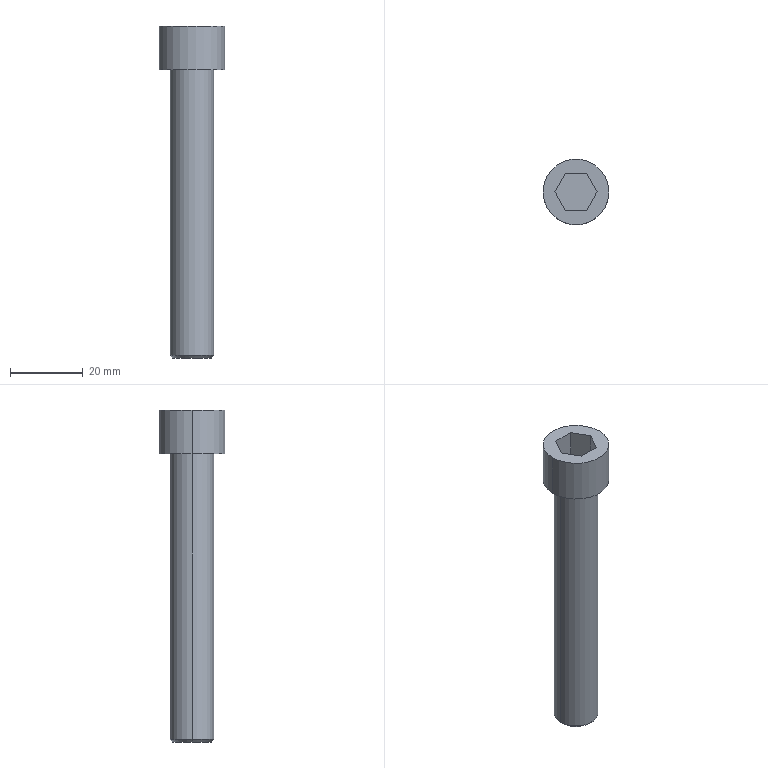Part | Creo | 1 solid | 16 faces | box 18 x 18 x 91 mm | volume 11293 mm3 | plane 10 | cylinder 4 | cone 2 | commonest cylinder face diameters 12 x2 18 x2
STEP:
#1=CARTESIAN_POINT('',(0.,0.,0.));
#2=DIRECTION('',(0.,0.,1.));
#3=DIRECTION('',(1.,0.,0.));
#4=AXIS2_PLACEMENT_3D('',#1,#2,#3);
#5=CARTESIAN_POINT('',(190.927,150.543,206.956));
#6=VERTEX_POINT('',#5);
#7=CARTESIAN_POINT('',(202.927,150.543,206.956));
#8=VERTEX_POINT('',#7);
#9=CARTESIAN_POINT('',(196.927,150.543,206.956));
#10=DIRECTION('',(0.,0.,-1.));
#11=DIRECTION('',(-1.,0.,0.));
#12=AXIS2_PLACEMENT_3D('',#9,#10,#11);
#13=CIRCLE('',#12,6.);
#14=EDGE_CURVE('',#6,#8,#13,.T.);
#15=ORIENTED_EDGE('',*,*,#14,.T.);
#16=CARTESIAN_POINT('',(202.927,150.543,285.245));
#17=VERTEX_POINT('',#16);
#18=CARTESIAN_POINT('',(202.927,150.543,285.245));
#19=DIRECTION('',(0.,0.,-1.));
#20=VECTOR('',#19,78.29);
#21=LINE('',#18,#20);
#22=EDGE_CURVE('',#17,#8,#21,.T.);
#23=ORIENTED_EDGE('',*,*,#22,.F.);
#24=CARTESIAN_POINT('',(190.927,150.543,285.245));
#25=VERTEX_POINT('',#24);
#26=CARTESIAN_POINT('',(196.927,150.543,285.245));
#27=DIRECTION('',(0.,0.,1.));
#28=DIRECTION('',(1.,0.,0.));
#29=AXIS2_PLACEMENT_3D('',#26,#27,#28);
#30=CIRCLE('',#29,6.);
#31=EDGE_CURVE('',#17,#25,#30,.T.);
#32=ORIENTED_EDGE('',*,*,#31,.T.);
#33=CARTESIAN_POINT('',(190.927,150.543,285.245));
#34=DIRECTION('',(0.,0.,-1.));
#35=VECTOR('',#34,78.29);
#36=LINE('',#33,#35);
#37=EDGE_CURVE('',#25,#6,#36,.T.);
#38=ORIENTED_EDGE('',*,*,#37,.T.);
#39=EDGE_LOOP('',(#15,#23,#32,#38));
#40=FACE_OUTER_BOUND('',#39,.F.);
#41=CARTESIAN_POINT('',(196.927,150.543,285.245));
#42=DIRECTION('',(0.,0.,-1.));
#43=DIRECTION('',(-1.,0.,0.));
#44=AXIS2_PLACEMENT_3D('',#41,#42,#43);
#45=CYLINDRICAL_SURFACE('',#44,6.);
#46=ADVANCED_FACE('',(#40),#45,.T.);
#47=CARTESIAN_POINT('',(191.637,150.543,206.245));
#48=VERTEX_POINT('',#47);
#49=CARTESIAN_POINT('',(202.216,150.543,206.245));
#50=VERTEX_POINT('',#49);
#51=CARTESIAN_POINT('',(196.927,150.543,206.245));
#52=DIRECTION('',(0.,0.,-1.));
#53=DIRECTION('',(-1.,0.,0.));
#54=AXIS2_PLACEMENT_3D('',#51,#52,#53);
#55=CIRCLE('',#54,5.29);
#56=EDGE_CURVE('',#48,#50,#55,.T.);
#57=ORIENTED_EDGE('',*,*,#56,.T.);
#58=CARTESIAN_POINT('',(202.216,150.543,206.245));
#59=DIRECTION('',(0.7071,0.,0.7071));
#60=VECTOR('',#59,1.005);
#61=LINE('',#58,#60);
#62=EDGE_CURVE('',#50,#8,#61,.T.);
#63=ORIENTED_EDGE('',*,*,#62,.T.);
#64=ORIENTED_EDGE('',*,*,#14,.F.);
#65=CARTESIAN_POINT('',(191.637,150.543,206.245));
#66=DIRECTION('',(-0.7071,0.,0.7071));
#67=VECTOR('',#66,1.005);
#68=LINE('',#65,#67);
#69=EDGE_CURVE('',#48,#6,#68,.T.);
#70=ORIENTED_EDGE('',*,*,#69,.F.);
#71=EDGE_LOOP('',(#57,#63,#64,#70));
#72=FACE_OUTER_BOUND('',#71,.F.);
#73=CARTESIAN_POINT('',(196.927,150.543,206.601));
#74=DIRECTION('',(0.,0.,1.));
#75=DIRECTION('',(1.,0.,0.));
#76=AXIS2_PLACEMENT_3D('',#73,#74,#75);
#77=CONICAL_SURFACE('',#76,5.645,45.);
#78=ADVANCED_FACE('',(#72),#77,.T.);
#79=CARTESIAN_POINT('',(196.927,150.543,206.245));
#80=DIRECTION('',(0.,0.,-1.));
#81=DIRECTION('',(1.,0.,0.));
#82=AXIS2_PLACEMENT_3D('',#79,#80,#81);
#83=CIRCLE('',#82,5.29);
#84=EDGE_CURVE('',#50,#48,#83,.T.);
#85=ORIENTED_EDGE('',*,*,#84,.F.);
#86=ORIENTED_EDGE('',*,*,#56,.F.);
#87=EDGE_LOOP('',(#85,#86));
#88=FACE_OUTER_BOUND('',#87,.F.);
#89=CARTESIAN_POINT('',(196.927,150.543,206.245));
#90=DIRECTION('',(0.,0.,1.));
#91=DIRECTION('',(1.,0.,0.));
#92=AXIS2_PLACEMENT_3D('',#89,#90,#91);
#93=PLANE('',#92);
#94=ADVANCED_FACE('',(#88),#93,.F.);
#95=ORIENTED_EDGE('',*,*,#84,.T.);
#96=ORIENTED_EDGE('',*,*,#69,.T.);
#97=CARTESIAN_POINT('',(196.927,150.543,206.956));
#98=DIRECTION('',(0.,0.,-1.));
#99=DIRECTION('',(1.,0.,0.));
#100=AXIS2_PLACEMENT_3D('',#97,#98,#99);
#101=CIRCLE('',#100,6.);
#102=EDGE_CURVE('',#8,#6,#101,.T.);
#103=ORIENTED_EDGE('',*,*,#102,.F.);
#104=ORIENTED_EDGE('',*,*,#62,.F.);
#105=EDGE_LOOP('',(#95,#96,#103,#104));
#106=FACE_OUTER_BOUND('',#105,.F.);
#107=CARTESIAN_POINT('',(196.927,150.543,206.601));
#108=DIRECTION('',(0.,0.,1.));
#109=DIRECTION('',(1.,0.,0.));
#110=AXIS2_PLACEMENT_3D('',#107,#108,#109);
#111=CONICAL_SURFACE('',#110,5.645,45.);
#112=ADVANCED_FACE('',(#106),#111,.T.);
#113=ORIENTED_EDGE('',*,*,#102,.T.);
#114=ORIENTED_EDGE('',*,*,#37,.F.);
#115=CARTESIAN_POINT('',(196.927,150.543,285.245));
#116=DIRECTION('',(0.,0.,1.));
#117=DIRECTION('',(-1.,0.,0.));
#118=AXIS2_PLACEMENT_3D('',#115,#116,#117);
#119=CIRCLE('',#118,6.);
#120=EDGE_CURVE('',#25,#17,#119,.T.);
#121=ORIENTED_EDGE('',*,*,#120,.T.);
#122=ORIENTED_EDGE('',*,*,#22,.T.);
#123=EDGE_LOOP('',(#113,#114,#121,#122));
#124=FACE_OUTER_BOUND('',#123,.F.);
#125=CARTESIAN_POINT('',(196.927,150.543,285.245));
#126=DIRECTION('',(0.,0.,-1.));
#127=DIRECTION('',(-1.,0.,0.));
#128=AXIS2_PLACEMENT_3D('',#125,#126,#127);
#129=CYLINDRICAL_SURFACE('',#128,6.);
#130=ADVANCED_FACE('',(#124),#129,.T.);
#131=CARTESIAN_POINT('',(205.927,150.543,285.245));
#132=VERTEX_POINT('',#131);
#133=CARTESIAN_POINT('',(187.927,150.543,285.245));
#134=VERTEX_POINT('',#133);
#135=CARTESIAN_POINT('',(196.927,150.543,285.245));
#136=DIRECTION('',(0.,0.,-1.));
#137=DIRECTION('',(1.,0.,0.));
#138=AXIS2_PLACEMENT_3D('',#135,#136,#137);
#139=CIRCLE('',#138,9.);
#140=EDGE_CURVE('',#132,#134,#139,.T.);
#141=ORIENTED_EDGE('',*,*,#140,.F.);
#142=CARTESIAN_POINT('',(196.927,150.543,285.245));
#143=DIRECTION('',(0.,0.,-1.));
#144=DIRECTION('',(-1.,0.,0.));
#145=AXIS2_PLACEMENT_3D('',#142,#143,#144);
#146=CIRCLE('',#145,9.);
#147=EDGE_CURVE('',#134,#132,#146,.T.);
#148=ORIENTED_EDGE('',*,*,#147,.F.);
#149=EDGE_LOOP('',(#141,#148));
#150=FACE_OUTER_BOUND('',#149,.F.);
#151=ORIENTED_EDGE('',*,*,#31,.F.);
#152=ORIENTED_EDGE('',*,*,#120,.F.);
#153=EDGE_LOOP('',(#151,#152));
#154=FACE_BOUND('',#153,.F.);
#155=CARTESIAN_POINT('',(196.927,150.543,285.245));
#156=DIRECTION('',(0.,0.,-1.));
#157=DIRECTION('',(-1.,0.,0.));
#158=AXIS2_PLACEMENT_3D('',#155,#156,#157);
#159=PLANE('',#158);
#160=ADVANCED_FACE('',(#150,#154),#159,.T.);
#161=CARTESIAN_POINT('',(187.927,150.543,297.245));
#162=VERTEX_POINT('',#161);
#163=CARTESIAN_POINT('',(205.927,150.543,297.245));
#164=VERTEX_POINT('',#163);
#165=CARTESIAN_POINT('',(196.927,150.543,297.245));
#166=DIRECTION('',(0.,0.,1.));
#167=DIRECTION('',(-1.,0.,0.));
#168=AXIS2_PLACEMENT_3D('',#165,#166,#167);
#169=CIRCLE('',#168,9.);
#170=EDGE_CURVE('',#162,#164,#169,.T.);
#171=ORIENTED_EDGE('',*,*,#170,.T.);
#172=CARTESIAN_POINT('',(205.927,150.543,285.245));
#173=DIRECTION('',(0.,0.,1.));
#174=VECTOR('',#173,12.);
#175=LINE('',#172,#174);
#176=EDGE_CURVE('',#132,#164,#175,.T.);
#177=ORIENTED_EDGE('',*,*,#176,.F.);
#178=ORIENTED_EDGE('',*,*,#140,.T.);
#179=CARTESIAN_POINT('',(187.927,150.543,285.245));
#180=DIRECTION('',(0.,0.,1.));
#181=VECTOR('',#180,12.);
#182=LINE('',#179,#181);
#183=EDGE_CURVE('',#134,#162,#182,.T.);
#184=ORIENTED_EDGE('',*,*,#183,.T.);
#185=EDGE_LOOP('',(#171,#177,#178,#184));
#186=FACE_OUTER_BOUND('',#185,.F.);
#187=CARTESIAN_POINT('',(196.927,150.543,285.245));
#188=DIRECTION('',(0.,0.,1.));
#189=DIRECTION('',(1.,0.,0.));
#190=AXIS2_PLACEMENT_3D('',#187,#188,#189);
#191=CYLINDRICAL_SURFACE('',#190,9.);
#192=ADVANCED_FACE('',(#186),#191,.T.);
#193=CARTESIAN_POINT('',(196.927,150.543,297.245));
#194=DIRECTION('',(0.,0.,1.));
#195=DIRECTION('',(1.,0.,0.));
#196=AXIS2_PLACEMENT_3D('',#193,#194,#195);
#197=CIRCLE('',#196,9.);
#198=EDGE_CURVE('',#164,#162,#197,.T.);
#199=ORIENTED_EDGE('',*,*,#198,.F.);
#200=ORIENTED_EDGE('',*,*,#170,.F.);
#201=EDGE_LOOP('',(#199,#200));
#202=FACE_OUTER_BOUND('',#201,.F.);
#203=CARTESIAN_POINT('',(199.813,145.543,297.245));
#204=VERTEX_POINT('',#203);
#205=CARTESIAN_POINT('',(194.04,145.543,297.245));
#206=VERTEX_POINT('',#205);
#207=CARTESIAN_POINT('',(199.813,145.543,297.245));
#208=DIRECTION('',(-1.,0.,0.));
#209=VECTOR('',#208,5.774);
#210=LINE('',#207,#209);
#211=EDGE_CURVE('',#204,#206,#210,.T.);
#212=ORIENTED_EDGE('',*,*,#211,.F.);
#213=CARTESIAN_POINT('',(202.7,150.543,297.245));
#214=VERTEX_POINT('',#213);
#215=CARTESIAN_POINT('',(202.7,150.543,297.245));
#216=DIRECTION('',(-0.5,-0.866,0.));
#217=VECTOR('',#216,5.774);
#218=LINE('',#215,#217);
#219=EDGE_CURVE('',#214,#204,#218,.T.);
#220=ORIENTED_EDGE('',*,*,#219,.F.);
#221=CARTESIAN_POINT('',(199.813,155.543,297.245));
#222=VERTEX_POINT('',#221);
#223=CARTESIAN_POINT('',(199.813,155.543,297.245));
#224=DIRECTION('',(0.5,-0.866,0.));
#225=VECTOR('',#224,5.774);
#226=LINE('',#223,#225);
#227=EDGE_CURVE('',#222,#214,#226,.T.);
#228=ORIENTED_EDGE('',*,*,#227,.F.);
#229=CARTESIAN_POINT('',(194.04,155.543,297.245));
#230=VERTEX_POINT('',#229);
#231=CARTESIAN_POINT('',(194.04,155.543,297.245));
#232=DIRECTION('',(1.,0.,0.));
#233=VECTOR('',#232,5.774);
#234=LINE('',#231,#233);
#235=EDGE_CURVE('',#230,#222,#234,.T.);
#236=ORIENTED_EDGE('',*,*,#235,.F.);
#237=CARTESIAN_POINT('',(191.153,150.543,297.245));
#238=VERTEX_POINT('',#237);
#239=CARTESIAN_POINT('',(191.153,150.543,297.245));
#240=DIRECTION('',(0.5,0.866,0.));
#241=VECTOR('',#240,5.774);
#242=LINE('',#239,#241);
#243=EDGE_CURVE('',#238,#230,#242,.T.);
#244=ORIENTED_EDGE('',*,*,#243,.F.);
#245=CARTESIAN_POINT('',(194.04,145.543,297.245));
#246=DIRECTION('',(-0.5,0.866,0.));
#247=VECTOR('',#246,5.774);
#248=LINE('',#245,#247);
#249=EDGE_CURVE('',#206,#238,#248,.T.);
#250=ORIENTED_EDGE('',*,*,#249,.F.);
#251=EDGE_LOOP('',(#212,#220,#228,#236,#244,#250));
#252=FACE_BOUND('',#251,.F.);
#253=CARTESIAN_POINT('',(196.927,150.543,297.245));
#254=DIRECTION('',(0.,0.,1.));
#255=DIRECTION('',(1.,0.,0.));
#256=AXIS2_PLACEMENT_3D('',#253,#254,#255);
#257=PLANE('',#256);
#258=ADVANCED_FACE('',(#202,#252),#257,.T.);
#259=ORIENTED_EDGE('',*,*,#211,.T.);
#260=CARTESIAN_POINT('',(194.04,145.543,289.325));
#261=VERTEX_POINT('',#260);
#262=CARTESIAN_POINT('',(194.04,145.543,297.245));
#263=DIRECTION('',(0.,0.,-1.));
#264=VECTOR('',#263,7.92);
#265=LINE('',#262,#264);
#266=EDGE_CURVE('',#206,#261,#265,.T.);
#267=ORIENTED_EDGE('',*,*,#266,.T.);
#268=CARTESIAN_POINT('',(199.813,145.543,289.325));
#269=VERTEX_POINT('',#268);
#270=CARTESIAN_POINT('',(199.813,145.543,289.325));
#271=DIRECTION('',(-1.,0.,0.));
#272=VECTOR('',#271,5.774);
#273=LINE('',#270,#272);
#274=EDGE_CURVE('',#269,#261,#273,.T.);
#275=ORIENTED_EDGE('',*,*,#274,.F.);
#276=CARTESIAN_POINT('',(199.813,145.543,297.245));
#277=DIRECTION('',(0.,0.,-1.));
#278=VECTOR('',#277,7.92);
#279=LINE('',#276,#278);
#280=EDGE_CURVE('',#204,#269,#279,.T.);
#281=ORIENTED_EDGE('',*,*,#280,.F.);
#282=EDGE_LOOP('',(#259,#267,#275,#281));
#283=FACE_OUTER_BOUND('',#282,.F.);
#284=CARTESIAN_POINT('',(194.04,145.543,289.325));
#285=DIRECTION('',(0.,-1.,0.));
#286=DIRECTION('',(0.,0.,-1.));
#287=AXIS2_PLACEMENT_3D('',#284,#285,#286);
#288=PLANE('',#287);
#289=ADVANCED_FACE('',(#283),#288,.F.);
#290=ORIENTED_EDGE('',*,*,#249,.T.);
#291=CARTESIAN_POINT('',(191.153,150.543,289.325));
#292=VERTEX_POINT('',#291);
#293=CARTESIAN_POINT('',(191.153,150.543,297.245));
#294=DIRECTION('',(0.,0.,-1.));
#295=VECTOR('',#294,7.92);
#296=LINE('',#293,#295);
#297=EDGE_CURVE('',#238,#292,#296,.T.);
#298=ORIENTED_EDGE('',*,*,#297,.T.);
#299=CARTESIAN_POINT('',(191.153,150.543,289.325));
#300=DIRECTION('',(0.5,-0.866,0.));
#301=VECTOR('',#300,5.774);
#302=LINE('',#299,#301);
#303=EDGE_CURVE('',#292,#261,#302,.T.);
#304=ORIENTED_EDGE('',*,*,#303,.T.);
#305=ORIENTED_EDGE('',*,*,#266,.F.);
#306=EDGE_LOOP('',(#290,#298,#304,#305));
#307=FACE_OUTER_BOUND('',#306,.F.);
#308=CARTESIAN_POINT('',(191.153,150.543,289.325));
#309=DIRECTION('',(-0.866,-0.5,0.));
#310=DIRECTION('',(0.5,-0.866,0.));
#311=AXIS2_PLACEMENT_3D('',#308,#309,#310);
#312=PLANE('',#311);
#313=ADVANCED_FACE('',(#307),#312,.F.);
#314=ORIENTED_EDGE('',*,*,#243,.T.);
#315=CARTESIAN_POINT('',(194.04,155.543,289.325));
#316=VERTEX_POINT('',#315);
#317=CARTESIAN_POINT('',(194.04,155.543,297.245));
#318=DIRECTION('',(0.,0.,-1.));
#319=VECTOR('',#318,7.92);
#320=LINE('',#317,#319);
#321=EDGE_CURVE('',#230,#316,#320,.T.);
#322=ORIENTED_EDGE('',*,*,#321,.T.);
#323=CARTESIAN_POINT('',(194.04,155.543,289.325));
#324=DIRECTION('',(-0.5,-0.866,0.));
#325=VECTOR('',#324,5.774);
#326=LINE('',#323,#325);
#327=EDGE_CURVE('',#316,#292,#326,.T.);
#328=ORIENTED_EDGE('',*,*,#327,.T.);
#329=ORIENTED_EDGE('',*,*,#297,.F.);
#330=EDGE_LOOP('',(#314,#322,#328,#329));
#331=FACE_OUTER_BOUND('',#330,.F.);
#332=CARTESIAN_POINT('',(194.04,155.543,289.325));
#333=DIRECTION('',(-0.866,0.5,0.));
#334=DIRECTION('',(-0.5,-0.866,0.));
#335=AXIS2_PLACEMENT_3D('',#332,#333,#334);
#336=PLANE('',#335);
#337=ADVANCED_FACE('',(#331),#336,.F.);
#338=ORIENTED_EDGE('',*,*,#235,.T.);
#339=CARTESIAN_POINT('',(199.813,155.543,289.325));
#340=VERTEX_POINT('',#339);
#341=CARTESIAN_POINT('',(199.813,155.543,297.245));
#342=DIRECTION('',(0.,0.,-1.));
#343=VECTOR('',#342,7.92);
#344=LINE('',#341,#343);
#345=EDGE_CURVE('',#222,#340,#344,.T.);
#346=ORIENTED_EDGE('',*,*,#345,.T.);
#347=CARTESIAN_POINT('',(194.04,155.543,289.325));
#348=DIRECTION('',(1.,0.,0.));
#349=VECTOR('',#348,5.774);
#350=LINE('',#347,#349);
#351=EDGE_CURVE('',#316,#340,#350,.T.);
#352=ORIENTED_EDGE('',*,*,#351,.F.);
#353=ORIENTED_EDGE('',*,*,#321,.F.);
#354=EDGE_LOOP('',(#338,#346,#352,#353));
#355=FACE_OUTER_BOUND('',#354,.F.);
#356=CARTESIAN_POINT('',(199.813,155.543,289.325));
#357=DIRECTION('',(0.,1.,0.));
#358=DIRECTION('',(0.,0.,1.));
#359=AXIS2_PLACEMENT_3D('',#356,#357,#358);
#360=PLANE('',#359);
#361=ADVANCED_FACE('',(#355),#360,.F.);
#362=ORIENTED_EDGE('',*,*,#227,.T.);
#363=CARTESIAN_POINT('',(202.7,150.543,289.325));
#364=VERTEX_POINT('',#363);
#365=CARTESIAN_POINT('',(202.7,150.543,297.245));
#366=DIRECTION('',(0.,0.,-1.));
#367=VECTOR('',#366,7.92);
#368=LINE('',#365,#367);
#369=EDGE_CURVE('',#214,#364,#368,.T.);
#370=ORIENTED_EDGE('',*,*,#369,.T.);
#371=CARTESIAN_POINT('',(202.7,150.543,289.325));
#372=DIRECTION('',(-0.5,0.866,0.));
#373=VECTOR('',#372,5.774);
#374=LINE('',#371,#373);
#375=EDGE_CURVE('',#364,#340,#374,.T.);
#376=ORIENTED_EDGE('',*,*,#375,.T.);
#377=ORIENTED_EDGE('',*,*,#345,.F.);
#378=EDGE_LOOP('',(#362,#370,#376,#377));
#379=FACE_OUTER_BOUND('',#378,.F.);
#380=CARTESIAN_POINT('',(202.7,150.543,289.325));
#381=DIRECTION('',(0.866,0.5,0.));
#382=DIRECTION('',(-0.5,0.866,0.));
#383=AXIS2_PLACEMENT_3D('',#380,#381,#382);
#384=PLANE('',#383);
#385=ADVANCED_FACE('',(#379),#384,.F.);
#386=ORIENTED_EDGE('',*,*,#219,.T.);
#387=ORIENTED_EDGE('',*,*,#280,.T.);
#388=CARTESIAN_POINT('',(199.813,145.543,289.325));
#389=DIRECTION('',(0.5,0.866,0.));
#390=VECTOR('',#389,5.774);
#391=LINE('',#388,#390);
#392=EDGE_CURVE('',#269,#364,#391,.T.);
#393=ORIENTED_EDGE('',*,*,#392,.T.);
#394=ORIENTED_EDGE('',*,*,#369,.F.);
#395=EDGE_LOOP('',(#386,#387,#393,#394));
#396=FACE_OUTER_BOUND('',#395,.F.);
#397=CARTESIAN_POINT('',(199.813,145.543,289.325));
#398=DIRECTION('',(0.866,-0.5,0.));
#399=DIRECTION('',(0.5,0.866,0.));
#400=AXIS2_PLACEMENT_3D('',#397,#398,#399);
#401=PLANE('',#400);
#402=ADVANCED_FACE('',(#396),#401,.F.);
#403=ORIENTED_EDGE('',*,*,#274,.T.);
#404=ORIENTED_EDGE('',*,*,#303,.F.);
#405=ORIENTED_EDGE('',*,*,#327,.F.);
#406=ORIENTED_EDGE('',*,*,#351,.T.);
#407=ORIENTED_EDGE('',*,*,#375,.F.);
#408=ORIENTED_EDGE('',*,*,#392,.F.);
#409=EDGE_LOOP('',(#403,#404,#405,#406,#407,#408));
#410=FACE_OUTER_BOUND('',#409,.F.);
#411=CARTESIAN_POINT('',(199.813,145.543,289.325));
#412=DIRECTION('',(0.,0.,1.));
#413=DIRECTION('',(1.,0.,0.));
#414=AXIS2_PLACEMENT_3D('',#411,#412,#413);
#415=PLANE('',#414);
#416=ADVANCED_FACE('',(#410),#415,.T.);
#417=ORIENTED_EDGE('',*,*,#198,.T.);
#418=ORIENTED_EDGE('',*,*,#183,.F.);
#419=ORIENTED_EDGE('',*,*,#147,.T.);
#420=ORIENTED_EDGE('',*,*,#176,.T.);
#421=EDGE_LOOP('',(#417,#418,#419,#420));
#422=FACE_OUTER_BOUND('',#421,.F.);
#423=CARTESIAN_POINT('',(196.927,150.543,285.245));
#424=DIRECTION('',(0.,0.,1.));
#425=DIRECTION('',(1.,0.,0.));
#426=AXIS2_PLACEMENT_3D('',#423,#424,#425);
#427=CYLINDRICAL_SURFACE('',#426,9.);
#428=ADVANCED_FACE('',(#422),#427,.T.);
#429=CLOSED_SHELL('',(#46,#78,#94,#112,#130,#160,#192,#258,#289,#313,#337,#361,#385,#402,#416,#428));
#430=MANIFOLD_SOLID_BREP('',#429);
#431=(LENGTH_UNIT()NAMED_UNIT(*)SI_UNIT(.MILLI.,.METRE.));
#432=UNCERTAINTY_MEASURE_WITH_UNIT(LENGTH_MEASURE(0.009449),#431,'','');
#433=(NAMED_UNIT(*)PLANE_ANGLE_UNIT()SI_UNIT($,.RADIAN.));
#434=PLANE_ANGLE_MEASURE_WITH_UNIT(PLANE_ANGLE_MEASURE(0.01745),#433);
#435=(CONVERSION_BASED_UNIT('DEGREE',#434)NAMED_UNIT(*)PLANE_ANGLE_UNIT());
#436=(NAMED_UNIT(*)SI_UNIT($,.STERADIAN.)SOLID_ANGLE_UNIT());
#437=(GEOMETRIC_REPRESENTATION_CONTEXT(3)GLOBAL_UNCERTAINTY_ASSIGNED_CONTEXT((#432))GLOBAL_UNIT_ASSIGNED_CONTEXT((#431,#435,#436))REPRESENTATION_CONTEXT('',''));
#438=ADVANCED_BREP_SHAPE_REPRESENTATION('',(#4,#430),#437);